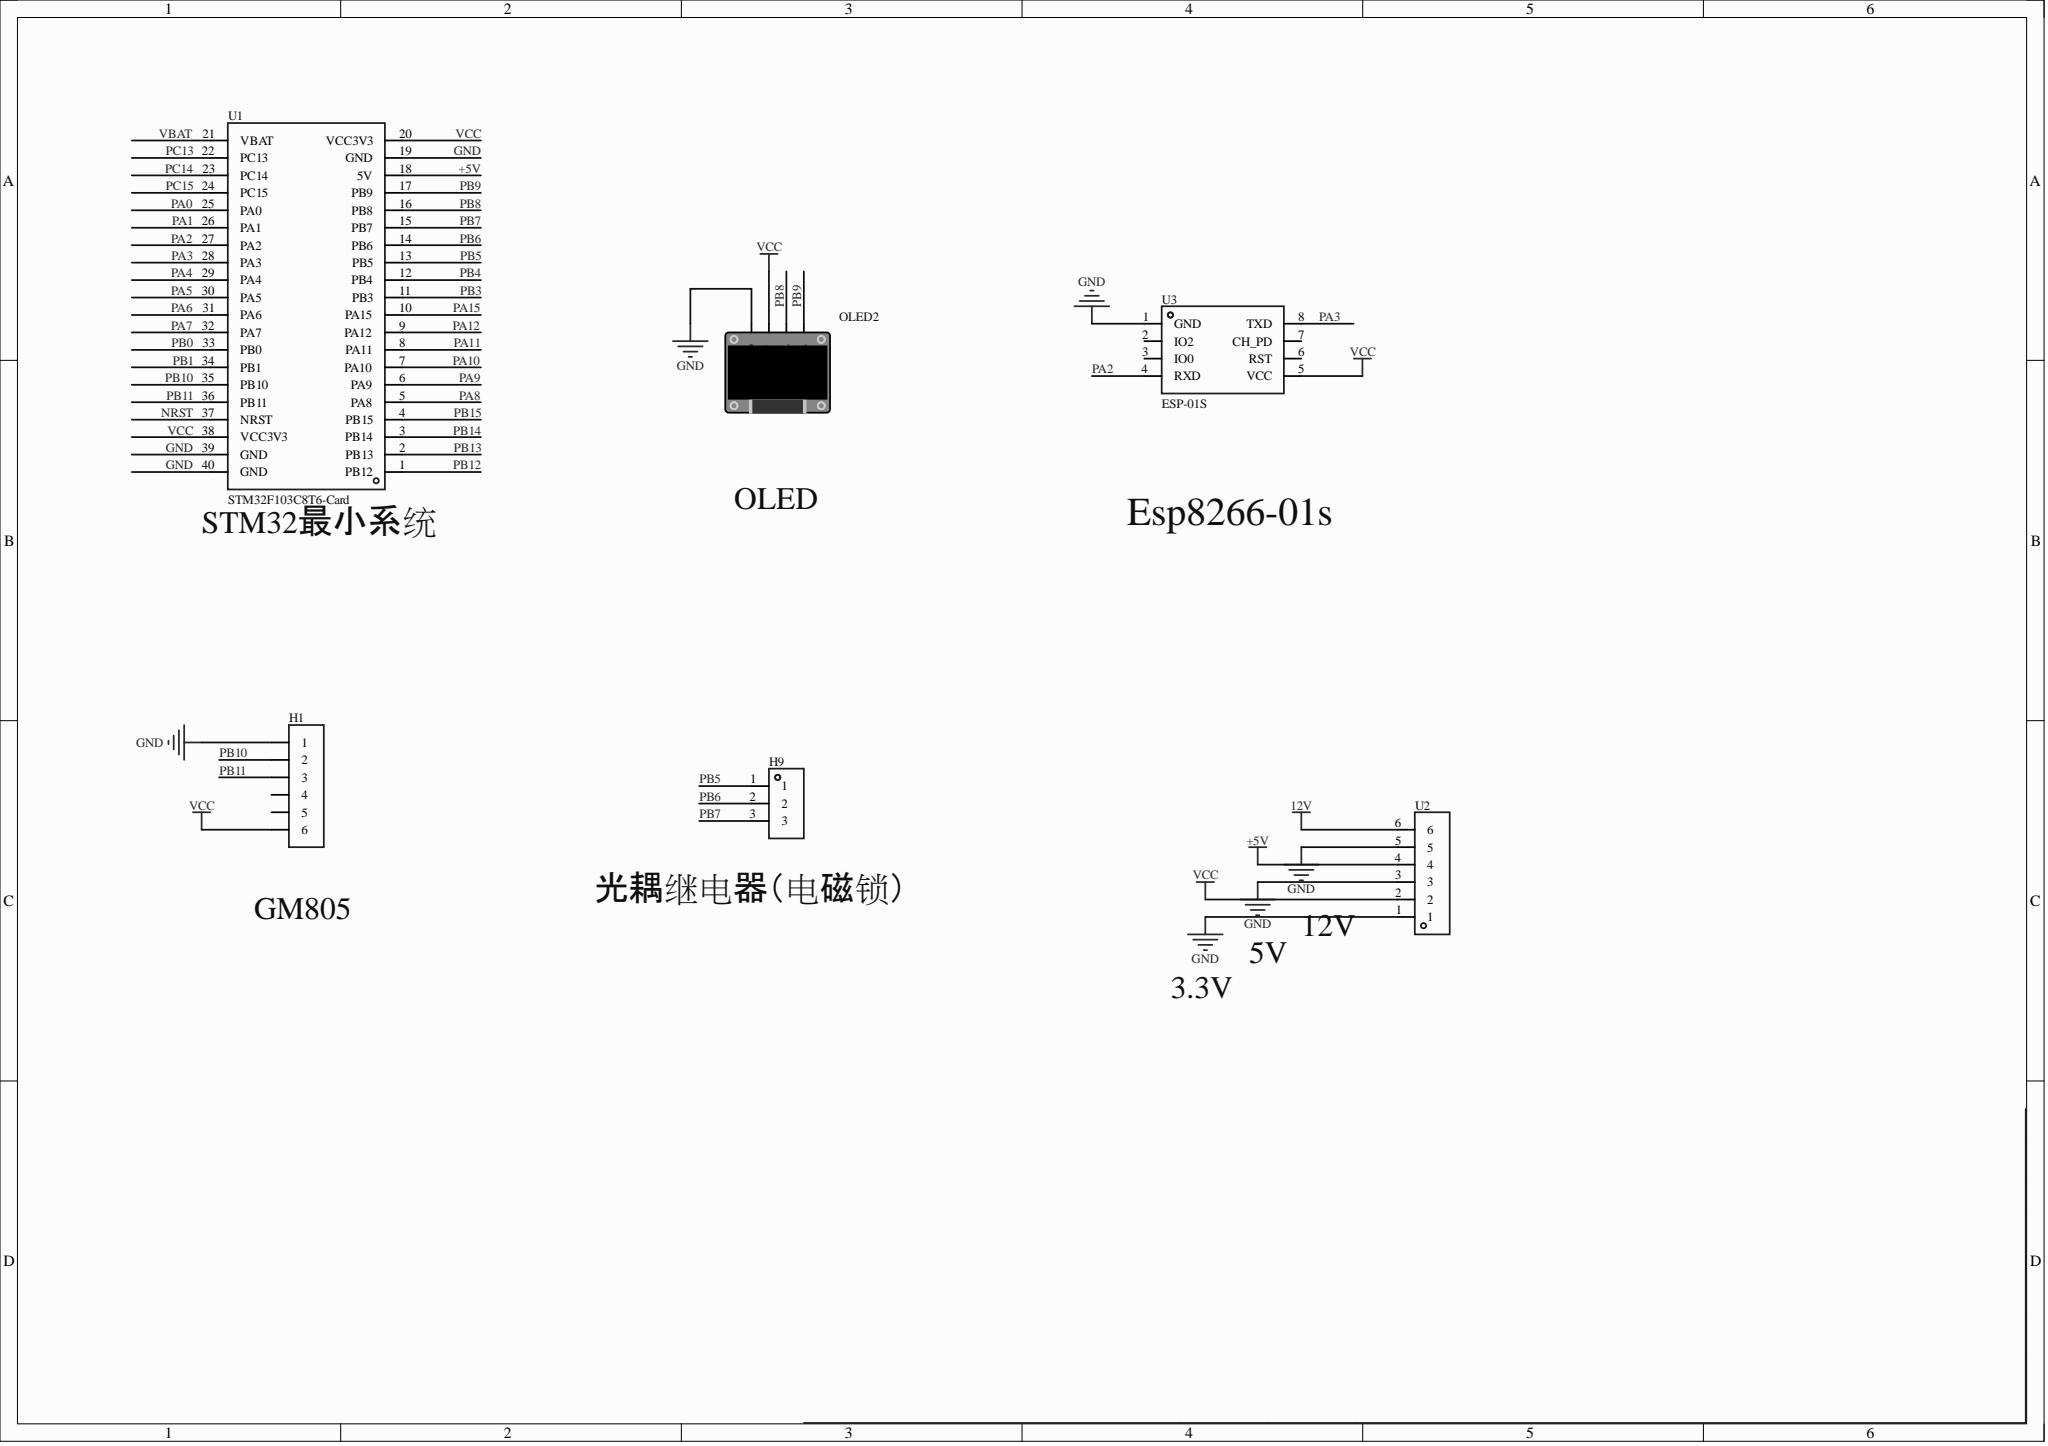Circuit board | Altium Designer | 6 parts | 12 nets
Bill of materials:
Comment,Description,Designator,Footprint,LibRef,Quantity
"","","H1","HDR-TH_6P-P2.54-V-M-1","HDR-M_2.54_1x6P","1"
"","","H9","HDR-TH_3P-P2.54-V-F","HDR-F_2.54_1x3P","1"
"","","OLED2","0.96OLED_4P","0.96OLED模块_4P","1"
"STM32F103C8T6-Card","","U1","CONN-TH_L53.3-W22.9_STM32F103C8T6-CARD","STM32F103C8T6-Card","1"
"LG128V 5.08 6P180度螺丝用十字带一字型","","U2","CONN-TH_6P-P5.00_LG128V","LG128V 5.08 6P180度螺丝用十字带一字型","1"
"ESP-01S","","U3","WIFIM-TH_ESP-01S","ESP-01S_C111009","1"
Netlist (Protel format):
[
H1
HDR-TH_6P-P2.54-V-M-1




]
[
H9
HDR-TH_3P-P2.54-V-F




]
[
OLED2
0.96OLED_4P




]
[
U1
CONN-TH_L53.3-W22.9_STM32F103C8T6-CARD
STM32F103C8T6-Card



]
[
U2
CONN-TH_6P-P5.00_LG128V
LG128V 5.08 6P180度螺丝用十字带一字型



]
[
U3
WIFIM-TH_ESP-01S
ESP-01S



]
(
VCC
H1-6
OLED2-2
U1-20
U1-38
U2-2
U3-5
)
(
PB11
H1-3
U1-36
)
(
PB10
H1-2
U1-35
)
(
PB9
OLED2-4
U1-17
)
(
PB8
OLED2-3
U1-16
)
(
PB7
H9-3
U1-15
)
(
PB6
H9-2
U1-14
)
(
PB5
H9-1
U1-13
)
(
PA3
U1-28
U3-8
)
(
PA2
U1-27
U3-4
)
(
GND
H1-1
OLED2-1
U1-19
U1-39
U1-40
U2-1
U2-3
U2-5
U3-1
)
(
+5V
U1-18
U2-4
)